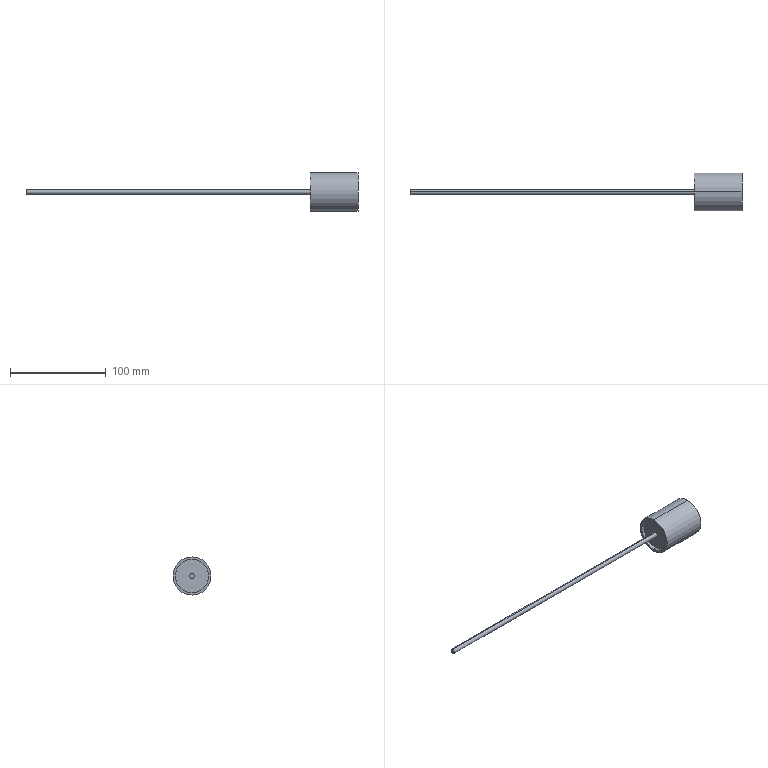Part | SolidWorks | features BaseBody 1, ICE 1 | 1 solid | 10 faces | box 347 x 40 x 40 mm | volume 65836 mm3 | cylinder 6 | plane 4 | commonest cylinder face diameters 5 x2 35 x2 40 x2
STEP:
#1=CARTESIAN_POINT('',(-369.28,0.,2.5));
#2=VERTEX_POINT('',#1);
#3=CARTESIAN_POINT('',(-369.28,0.,-2.5));
#4=VERTEX_POINT('',#3);
#5=CARTESIAN_POINT('',(-369.28,0.,0.));
#6=DIRECTION('',(-1.,0.,0.));
#7=DIRECTION('',(0.,0.,1.));
#8=AXIS2_PLACEMENT_3D('',#5,#6,#7);
#9=CIRCLE('',#8,2.5);
#10=EDGE_CURVE('',#2,#4,#9,.T.);
#11=ORIENTED_EDGE('',*,*,#10,.F.);
#12=CARTESIAN_POINT('',(-69.28,0.,2.5));
#13=VERTEX_POINT('',#12);
#14=CARTESIAN_POINT('',(-369.28,0.,2.5));
#15=DIRECTION('',(1.,0.,0.));
#16=VECTOR('',#15,1000.);
#17=LINE('',#14,#16);
#18=EDGE_CURVE('',#2,#13,#17,.T.);
#19=ORIENTED_EDGE('',*,*,#18,.T.);
#20=CARTESIAN_POINT('',(-69.28,0.,-2.5));
#21=VERTEX_POINT('',#20);
#22=CARTESIAN_POINT('',(-69.28,0.,0.));
#23=DIRECTION('',(-1.,0.,0.));
#24=DIRECTION('',(0.,0.,-1.));
#25=AXIS2_PLACEMENT_3D('',#22,#23,#24);
#26=CIRCLE('',#25,2.5);
#27=EDGE_CURVE('',#13,#21,#26,.T.);
#28=ORIENTED_EDGE('',*,*,#27,.T.);
#29=CARTESIAN_POINT('',(-369.28,0.,-2.5));
#30=DIRECTION('',(1.,0.,0.));
#31=VECTOR('',#30,1000.);
#32=LINE('',#29,#31);
#33=EDGE_CURVE('',#4,#21,#32,.T.);
#34=ORIENTED_EDGE('',*,*,#33,.F.);
#35=EDGE_LOOP('',(#11,#19,#28,#34));
#36=FACE_OUTER_BOUND('',#35,.T.);
#37=CARTESIAN_POINT('',(-369.28,0.,0.));
#38=DIRECTION('',(1.,0.,0.));
#39=DIRECTION('',(0.,0.,-1.));
#40=AXIS2_PLACEMENT_3D('',#37,#38,#39);
#41=CYLINDRICAL_SURFACE('',#40,2.5);
#42=ADVANCED_FACE('',(#36),#41,.T.);
#43=CARTESIAN_POINT('',(-22.28,0.,20.));
#44=VERTEX_POINT('',#43);
#45=CARTESIAN_POINT('',(-22.28,0.,-20.));
#46=VERTEX_POINT('',#45);
#47=CARTESIAN_POINT('',(-22.28,0.,0.));
#48=DIRECTION('',(-1.,0.,0.));
#49=DIRECTION('',(0.,0.,1.));
#50=AXIS2_PLACEMENT_3D('',#47,#48,#49);
#51=CIRCLE('',#50,20.);
#52=EDGE_CURVE('',#44,#46,#51,.T.);
#53=ORIENTED_EDGE('',*,*,#52,.T.);
#54=CARTESIAN_POINT('',(-72.28,0.,-20.));
#55=VERTEX_POINT('',#54);
#56=CARTESIAN_POINT('',(-122.204,0.,-20.));
#57=DIRECTION('',(-1.,0.,0.));
#58=VECTOR('',#57,1000.);
#59=LINE('',#56,#58);
#60=EDGE_CURVE('',#46,#55,#59,.T.);
#61=ORIENTED_EDGE('',*,*,#60,.T.);
#62=CARTESIAN_POINT('',(-72.28,0.,20.));
#63=VERTEX_POINT('',#62);
#64=CARTESIAN_POINT('',(-72.28,0.,0.));
#65=DIRECTION('',(1.,0.,0.));
#66=DIRECTION('',(0.,0.,1.));
#67=AXIS2_PLACEMENT_3D('',#64,#65,#66);
#68=CIRCLE('',#67,20.);
#69=EDGE_CURVE('',#55,#63,#68,.T.);
#70=ORIENTED_EDGE('',*,*,#69,.T.);
#71=CARTESIAN_POINT('',(-122.204,0.,20.));
#72=DIRECTION('',(-1.,0.,0.));
#73=VECTOR('',#72,1000.);
#74=LINE('',#71,#73);
#75=EDGE_CURVE('',#44,#63,#74,.T.);
#76=ORIENTED_EDGE('',*,*,#75,.F.);
#77=EDGE_LOOP('',(#53,#61,#70,#76));
#78=FACE_OUTER_BOUND('',#77,.T.);
#79=CARTESIAN_POINT('',(-122.204,0.,0.));
#80=DIRECTION('',(-1.,0.,0.));
#81=DIRECTION('',(0.,0.,1.));
#82=AXIS2_PLACEMENT_3D('',#79,#80,#81);
#83=CYLINDRICAL_SURFACE('',#82,20.);
#84=ADVANCED_FACE('',(#78),#83,.T.);
#85=CARTESIAN_POINT('',(-69.28,0.,-17.5));
#86=VERTEX_POINT('',#85);
#87=CARTESIAN_POINT('',(-69.28,0.,17.5));
#88=VERTEX_POINT('',#87);
#89=CARTESIAN_POINT('',(-69.28,0.,0.));
#90=DIRECTION('',(-1.,0.,0.));
#91=DIRECTION('',(0.,0.,1.));
#92=AXIS2_PLACEMENT_3D('',#89,#90,#91);
#93=CIRCLE('',#92,17.5);
#94=EDGE_CURVE('',#86,#88,#93,.T.);
#95=ORIENTED_EDGE('',*,*,#94,.F.);
#96=CARTESIAN_POINT('',(-72.28,0.,-17.5));
#97=VERTEX_POINT('',#96);
#98=CARTESIAN_POINT('',(-122.204,0.,-17.5));
#99=DIRECTION('',(-1.,0.,0.));
#100=VECTOR('',#99,1000.);
#101=LINE('',#98,#100);
#102=EDGE_CURVE('',#86,#97,#101,.T.);
#103=ORIENTED_EDGE('',*,*,#102,.T.);
#104=CARTESIAN_POINT('',(-72.28,0.,17.5));
#105=VERTEX_POINT('',#104);
#106=CARTESIAN_POINT('',(-72.28,0.,0.));
#107=DIRECTION('',(-1.,0.,0.));
#108=DIRECTION('',(0.,0.,1.));
#109=AXIS2_PLACEMENT_3D('',#106,#107,#108);
#110=CIRCLE('',#109,17.5);
#111=EDGE_CURVE('',#97,#105,#110,.T.);
#112=ORIENTED_EDGE('',*,*,#111,.T.);
#113=CARTESIAN_POINT('',(-122.204,0.,17.5));
#114=DIRECTION('',(-1.,0.,0.));
#115=VECTOR('',#114,1000.);
#116=LINE('',#113,#115);
#117=EDGE_CURVE('',#88,#105,#116,.T.);
#118=ORIENTED_EDGE('',*,*,#117,.F.);
#119=EDGE_LOOP('',(#95,#103,#112,#118));
#120=FACE_OUTER_BOUND('',#119,.T.);
#121=CARTESIAN_POINT('',(-122.204,0.,0.));
#122=DIRECTION('',(-1.,0.,0.));
#123=DIRECTION('',(0.,0.,1.));
#124=AXIS2_PLACEMENT_3D('',#121,#122,#123);
#125=CYLINDRICAL_SURFACE('',#124,17.5);
#126=ADVANCED_FACE('',(#120),#125,.F.);
#127=ORIENTED_EDGE('',*,*,#60,.F.);
#128=CARTESIAN_POINT('',(-22.28,0.,0.));
#129=DIRECTION('',(-1.,0.,0.));
#130=DIRECTION('',(0.,0.,1.));
#131=AXIS2_PLACEMENT_3D('',#128,#129,#130);
#132=CIRCLE('',#131,20.);
#133=EDGE_CURVE('',#46,#44,#132,.T.);
#134=ORIENTED_EDGE('',*,*,#133,.T.);
#135=ORIENTED_EDGE('',*,*,#75,.T.);
#136=CARTESIAN_POINT('',(-72.28,0.,0.));
#137=DIRECTION('',(1.,0.,0.));
#138=DIRECTION('',(0.,0.,1.));
#139=AXIS2_PLACEMENT_3D('',#136,#137,#138);
#140=CIRCLE('',#139,20.);
#141=EDGE_CURVE('',#63,#55,#140,.T.);
#142=ORIENTED_EDGE('',*,*,#141,.T.);
#143=EDGE_LOOP('',(#127,#134,#135,#142));
#144=FACE_OUTER_BOUND('',#143,.T.);
#145=CARTESIAN_POINT('',(-122.204,0.,0.));
#146=DIRECTION('',(-1.,0.,0.));
#147=DIRECTION('',(0.,0.,1.));
#148=AXIS2_PLACEMENT_3D('',#145,#146,#147);
#149=CYLINDRICAL_SURFACE('',#148,20.);
#150=ADVANCED_FACE('',(#144),#149,.T.);
#151=ORIENTED_EDGE('',*,*,#141,.F.);
#152=ORIENTED_EDGE('',*,*,#69,.F.);
#153=EDGE_LOOP('',(#151,#152));
#154=FACE_OUTER_BOUND('',#153,.T.);
#155=CARTESIAN_POINT('',(-72.28,0.,0.));
#156=DIRECTION('',(-1.,0.,0.));
#157=DIRECTION('',(0.,0.,1.));
#158=AXIS2_PLACEMENT_3D('',#155,#156,#157);
#159=CIRCLE('',#158,17.5);
#160=EDGE_CURVE('',#105,#97,#159,.T.);
#161=ORIENTED_EDGE('',*,*,#160,.F.);
#162=ORIENTED_EDGE('',*,*,#111,.F.);
#163=EDGE_LOOP('',(#161,#162));
#164=FACE_BOUND('',#163,.T.);
#165=CARTESIAN_POINT('',(-72.28,20.,0.));
#166=DIRECTION('',(1.,0.,0.));
#167=DIRECTION('',(0.,0.,-1.));
#168=AXIS2_PLACEMENT_3D('',#165,#166,#167);
#169=PLANE('',#168);
#170=ADVANCED_FACE('',(#154,#164),#169,.F.);
#171=ORIENTED_EDGE('',*,*,#52,.F.);
#172=ORIENTED_EDGE('',*,*,#133,.F.);
#173=EDGE_LOOP('',(#171,#172));
#174=FACE_OUTER_BOUND('',#173,.T.);
#175=CARTESIAN_POINT('',(-22.28,20.,0.));
#176=DIRECTION('',(-1.,0.,0.));
#177=DIRECTION('',(0.,0.,1.));
#178=AXIS2_PLACEMENT_3D('',#175,#176,#177);
#179=PLANE('',#178);
#180=ADVANCED_FACE('',(#174),#179,.F.);
#181=ORIENTED_EDGE('',*,*,#102,.F.);
#182=CARTESIAN_POINT('',(-69.28,0.,0.));
#183=DIRECTION('',(-1.,0.,0.));
#184=DIRECTION('',(0.,0.,1.));
#185=AXIS2_PLACEMENT_3D('',#182,#183,#184);
#186=CIRCLE('',#185,17.5);
#187=EDGE_CURVE('',#88,#86,#186,.T.);
#188=ORIENTED_EDGE('',*,*,#187,.F.);
#189=ORIENTED_EDGE('',*,*,#117,.T.);
#190=ORIENTED_EDGE('',*,*,#160,.T.);
#191=EDGE_LOOP('',(#181,#188,#189,#190));
#192=FACE_OUTER_BOUND('',#191,.T.);
#193=CARTESIAN_POINT('',(-122.204,0.,0.));
#194=DIRECTION('',(-1.,0.,0.));
#195=DIRECTION('',(0.,0.,1.));
#196=AXIS2_PLACEMENT_3D('',#193,#194,#195);
#197=CYLINDRICAL_SURFACE('',#196,17.5);
#198=ADVANCED_FACE('',(#192),#197,.F.);
#199=CARTESIAN_POINT('',(-69.28,0.,0.));
#200=DIRECTION('',(-1.,0.,0.));
#201=DIRECTION('',(0.,0.,-1.));
#202=AXIS2_PLACEMENT_3D('',#199,#200,#201);
#203=CIRCLE('',#202,2.5);
#204=EDGE_CURVE('',#21,#13,#203,.T.);
#205=ORIENTED_EDGE('',*,*,#204,.F.);
#206=ORIENTED_EDGE('',*,*,#27,.F.);
#207=EDGE_LOOP('',(#205,#206));
#208=FACE_BOUND('',#207,.T.);
#209=ORIENTED_EDGE('',*,*,#187,.T.);
#210=ORIENTED_EDGE('',*,*,#94,.T.);
#211=EDGE_LOOP('',(#209,#210));
#212=FACE_OUTER_BOUND('',#211,.T.);
#213=CARTESIAN_POINT('',(-69.28,0.,0.));
#214=DIRECTION('',(1.,0.,0.));
#215=DIRECTION('',(0.,0.,-1.));
#216=AXIS2_PLACEMENT_3D('',#213,#214,#215);
#217=PLANE('',#216);
#218=ADVANCED_FACE('',(#208,#212),#217,.F.);
#219=ORIENTED_EDGE('',*,*,#18,.F.);
#220=CARTESIAN_POINT('',(-369.28,0.,0.));
#221=DIRECTION('',(-1.,0.,0.));
#222=DIRECTION('',(0.,0.,1.));
#223=AXIS2_PLACEMENT_3D('',#220,#221,#222);
#224=CIRCLE('',#223,2.5);
#225=EDGE_CURVE('',#4,#2,#224,.T.);
#226=ORIENTED_EDGE('',*,*,#225,.F.);
#227=ORIENTED_EDGE('',*,*,#33,.T.);
#228=ORIENTED_EDGE('',*,*,#204,.T.);
#229=EDGE_LOOP('',(#219,#226,#227,#228));
#230=FACE_OUTER_BOUND('',#229,.T.);
#231=CARTESIAN_POINT('',(-369.28,0.,0.));
#232=DIRECTION('',(1.,0.,0.));
#233=DIRECTION('',(0.,0.,-1.));
#234=AXIS2_PLACEMENT_3D('',#231,#232,#233);
#235=CYLINDRICAL_SURFACE('',#234,2.5);
#236=ADVANCED_FACE('',(#230),#235,.T.);
#237=ORIENTED_EDGE('',*,*,#225,.T.);
#238=ORIENTED_EDGE('',*,*,#10,.T.);
#239=EDGE_LOOP('',(#237,#238));
#240=FACE_OUTER_BOUND('',#239,.T.);
#241=CARTESIAN_POINT('',(-369.28,0.,0.));
#242=DIRECTION('',(-1.,0.,0.));
#243=DIRECTION('',(0.,0.,1.));
#244=AXIS2_PLACEMENT_3D('',#241,#242,#243);
#245=PLANE('',#244);
#246=ADVANCED_FACE('',(#240),#245,.T.);
#247=CLOSED_SHELL('',(#42,#84,#126,#150,#170,#180,#198,#218,#236,#246));
#248=MANIFOLD_SOLID_BREP('',#247);
#249=CARTESIAN_POINT('',(0.,0.,0.));
#250=DIRECTION('',(0.,0.,1.));
#251=DIRECTION('',(1.,0.,0.));
#252=AXIS2_PLACEMENT_3D('',#249,#250,#251);
#253=(LENGTH_UNIT()NAMED_UNIT(*)SI_UNIT(.MILLI.,.METRE.));
#254=UNCERTAINTY_MEASURE_WITH_UNIT(LENGTH_MEASURE(0.00001),#253,'','');
#255=(NAMED_UNIT(*)PLANE_ANGLE_UNIT()SI_UNIT($,.RADIAN.));
#256=(NAMED_UNIT(*)SI_UNIT($,.STERADIAN.)SOLID_ANGLE_UNIT());
#257=(GEOMETRIC_REPRESENTATION_CONTEXT(3)GLOBAL_UNCERTAINTY_ASSIGNED_CONTEXT((#254))GLOBAL_UNIT_ASSIGNED_CONTEXT((#253,#255,#256))REPRESENTATION_CONTEXT('',''));
#258=ADVANCED_BREP_SHAPE_REPRESENTATION('',(#248,#252),#257);